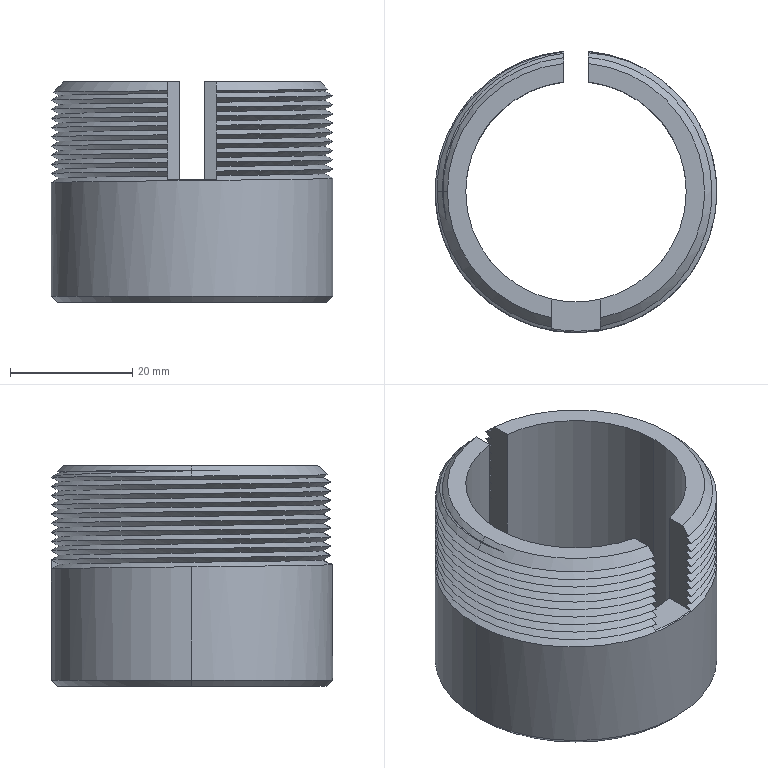Part | SolidWorks | features Chamfer 2, ICE 2, Extrusion 1, Helix 1, SweepCut 1 | 1 solid | 63 faces | box 46 x 45.913 x 36 mm | volume 20268 mm3 | spline 41 | cone 8 | plane 8 | cylinder 6 | commonest cylinder face diameters 36 x3 46 x3